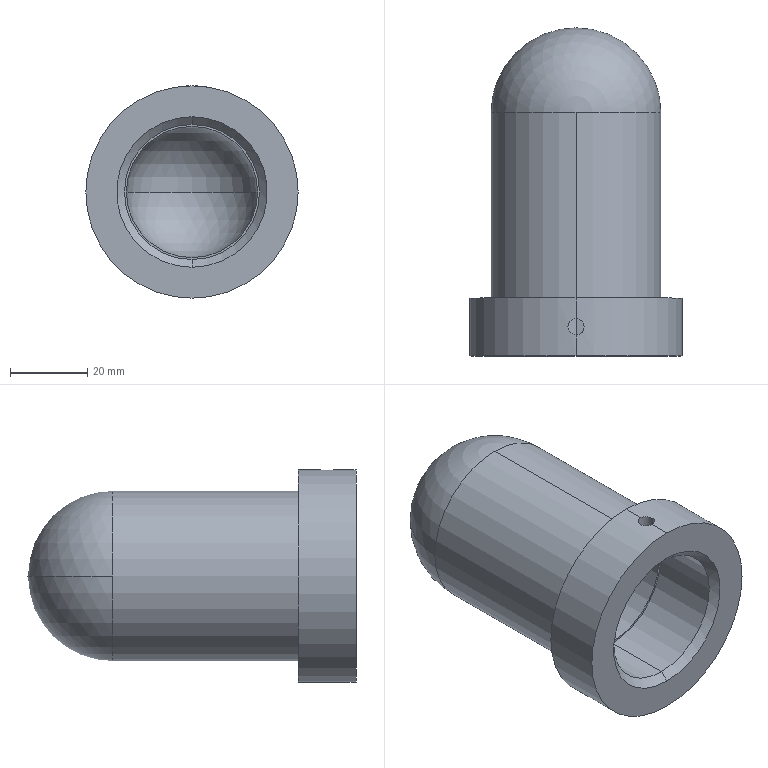Part | SolidWorks | features 3DProfileFeature 1, Chamfer 1, HoleWzd 1, Revolution 1 | 1 solid | 19 faces | box 55 x 85 x 55 mm | volume 61984 mm3 | cylinder 10 | sphere 4 | plane 3 | cone 2 | commonest cylinder face diameters 4.2 x2 34 x2 35 x2 44 x2 55 x2
STEP:
#1=CARTESIAN_POINT('',(0.,2.,17.5));
#2=VERTEX_POINT('',#1);
#3=CARTESIAN_POINT('',(0.,2.,-17.5));
#4=VERTEX_POINT('',#3);
#5=CARTESIAN_POINT('',(0.,2.,0.));
#6=DIRECTION('',(0.,-1.,0.));
#7=DIRECTION('',(0.,0.,1.));
#8=AXIS2_PLACEMENT_3D('',#5,#6,#7);
#9=CIRCLE('',#8,17.5);
#10=EDGE_CURVE('',#2,#4,#9,.T.);
#11=ORIENTED_EDGE('',*,*,#10,.F.);
#12=CARTESIAN_POINT('',(0.,0.,19.5));
#13=VERTEX_POINT('',#12);
#14=CARTESIAN_POINT('',(0.,2.,17.5));
#15=DIRECTION('',(0.,-0.7071,0.7071));
#16=VECTOR('',#15,1000.);
#17=LINE('',#14,#16);
#18=EDGE_CURVE('',#2,#13,#17,.T.);
#19=ORIENTED_EDGE('',*,*,#18,.T.);
#20=CARTESIAN_POINT('',(0.,0.,-19.5));
#21=VERTEX_POINT('',#20);
#22=CARTESIAN_POINT('',(0.,0.,0.));
#23=DIRECTION('',(0.,1.,0.));
#24=DIRECTION('',(0.,0.,1.));
#25=AXIS2_PLACEMENT_3D('',#22,#23,#24);
#26=CIRCLE('',#25,19.5);
#27=EDGE_CURVE('',#21,#13,#26,.T.);
#28=ORIENTED_EDGE('',*,*,#27,.F.);
#29=CARTESIAN_POINT('',(0.,2.,-17.5));
#30=DIRECTION('',(0.,-0.7071,-0.7071));
#31=VECTOR('',#30,1000.);
#32=LINE('',#29,#31);
#33=EDGE_CURVE('',#4,#21,#32,.T.);
#34=ORIENTED_EDGE('',*,*,#33,.F.);
#35=EDGE_LOOP('',(#11,#19,#28,#34));
#36=FACE_OUTER_BOUND('',#35,.T.);
#37=CARTESIAN_POINT('',(0.,2.,0.));
#38=DIRECTION('',(0.,-1.,0.));
#39=DIRECTION('',(0.,0.,-1.));
#40=AXIS2_PLACEMENT_3D('',#37,#38,#39);
#41=CONICAL_SURFACE('',#40,17.5,0.7854);
#42=ADVANCED_FACE('',(#36),#41,.F.);
#43=CARTESIAN_POINT('',(-2.101,7.524,17.373));
#44=VERTEX_POINT('',#43);
#45=CARTESIAN_POINT('',(0.,5.424,17.5));
#46=VERTEX_POINT('',#45);
#47=CARTESIAN_POINT('',(-2.101,7.524,17.373));
#48=CARTESIAN_POINT('',(-2.101,7.25,17.373));
#49=CARTESIAN_POINT('',(-2.046,6.973,17.38));
#50=CARTESIAN_POINT('',(-1.837,6.467,17.404));
#51=CARTESIAN_POINT('',(-1.68,6.233,17.42));
#52=CARTESIAN_POINT('',(-1.389,5.942,17.445));
#53=CARTESIAN_POINT('',(-1.281,5.854,17.453));
#54=CARTESIAN_POINT('',(-1.053,5.701,17.469));
#55=CARTESIAN_POINT('',(-0.9324,5.637,17.476));
#56=CARTESIAN_POINT('',(-0.6779,5.531,17.487));
#57=CARTESIAN_POINT('',(-0.5444,5.491,17.492));
#58=CARTESIAN_POINT('',(-0.2756,5.438,17.498));
#59=CARTESIAN_POINT('',(-0.1389,5.424,17.5));
#60=CARTESIAN_POINT('',(0.,5.424,17.5));
#61=B_SPLINE_CURVE_WITH_KNOTS('',3,(#47,#48,#49,#50,#51,#52,#53,#54,#55,#56,#57,#58,#59,#60),.UNSPECIFIED.,.F.,.F.,(4,2,2,2,2,2,4),(0.006571,0.007393,0.008215,0.008626,0.009037,0.009448,0.009859),.UNSPECIFIED.);
#62=EDGE_CURVE('',#44,#46,#61,.T.);
#63=ORIENTED_EDGE('',*,*,#62,.F.);
#64=CARTESIAN_POINT('',(-2.102,7.524,27.42));
#65=VERTEX_POINT('',#64);
#66=CARTESIAN_POINT('',(-2.102,7.524,27.5));
#67=DIRECTION('',(-0.00007928,0.,1.));
#68=VECTOR('',#67,1000.);
#69=LINE('',#66,#68);
#70=EDGE_CURVE('',#44,#65,#69,.T.);
#71=ORIENTED_EDGE('',*,*,#70,.T.);
#72=CARTESIAN_POINT('',(0.,5.424,27.5));
#73=VERTEX_POINT('',#72);
#74=CARTESIAN_POINT('',(0.,5.424,27.5));
#75=CARTESIAN_POINT('',(-0.1371,5.424,27.5));
#76=CARTESIAN_POINT('',(-0.2763,5.438,27.499));
#77=CARTESIAN_POINT('',(-0.5459,5.491,27.495));
#78=CARTESIAN_POINT('',(-0.6769,5.531,27.492));
#79=CARTESIAN_POINT('',(-0.9314,5.636,27.485));
#80=CARTESIAN_POINT('',(-1.054,5.702,27.48));
#81=CARTESIAN_POINT('',(-1.282,5.854,27.47));
#82=CARTESIAN_POINT('',(-1.388,5.94,27.465));
#83=CARTESIAN_POINT('',(-1.584,6.136,27.454));
#84=CARTESIAN_POINT('',(-1.671,6.243,27.449));
#85=CARTESIAN_POINT('',(-1.824,6.47,27.44));
#86=CARTESIAN_POINT('',(-1.889,6.593,27.435));
#87=CARTESIAN_POINT('',(-1.995,6.847,27.428));
#88=CARTESIAN_POINT('',(-2.035,6.978,27.425));
#89=CARTESIAN_POINT('',(-2.088,7.248,27.421));
#90=CARTESIAN_POINT('',(-2.102,7.387,27.42));
#91=CARTESIAN_POINT('',(-2.102,7.524,27.42));
#92=B_SPLINE_CURVE_WITH_KNOTS('',3,(#74,#75,#76,#77,#78,#79,#80,#81,#82,#83,#84,#85,#86,#87,#88,#89,#90,#91),.UNSPECIFIED.,.F.,.F.,(4,2,2,2,2,2,2,2,4),(0.003283,0.003693,0.004104,0.004515,0.004925,0.005336,0.005747,0.006157,0.006568),.UNSPECIFIED.);
#93=EDGE_CURVE('',#73,#65,#92,.T.);
#94=ORIENTED_EDGE('',*,*,#93,.F.);
#95=CARTESIAN_POINT('',(2.098,7.524,27.42));
#96=VERTEX_POINT('',#95);
#97=CARTESIAN_POINT('',(2.098,7.524,27.42));
#98=CARTESIAN_POINT('',(2.098,7.385,27.42));
#99=CARTESIAN_POINT('',(2.084,7.249,27.421));
#100=CARTESIAN_POINT('',(2.031,6.981,27.425));
#101=CARTESIAN_POINT('',(1.991,6.847,27.428));
#102=CARTESIAN_POINT('',(1.885,6.593,27.435));
#103=CARTESIAN_POINT('',(1.821,6.472,27.44));
#104=CARTESIAN_POINT('',(1.668,6.244,27.449));
#105=CARTESIAN_POINT('',(1.58,6.136,27.455));
#106=CARTESIAN_POINT('',(1.289,5.846,27.47));
#107=CARTESIAN_POINT('',(1.055,5.689,27.481));
#108=CARTESIAN_POINT('',(0.5502,5.48,27.496));
#109=CARTESIAN_POINT('',(0.2739,5.424,27.5));
#110=CARTESIAN_POINT('',(0.,5.424,27.5));
#111=B_SPLINE_CURVE_WITH_KNOTS('',3,(#97,#98,#99,#100,#101,#102,#103,#104,#105,#106,#107,#108,#109,#110),.UNSPECIFIED.,.F.,.F.,(4,2,2,2,2,2,4),(0.,0.0004103,0.0008206,0.001231,0.001641,0.002462,0.003283),.UNSPECIFIED.);
#112=EDGE_CURVE('',#96,#73,#111,.T.);
#113=ORIENTED_EDGE('',*,*,#112,.F.);
#114=CARTESIAN_POINT('',(2.099,7.524,17.374));
#115=VERTEX_POINT('',#114);
#116=CARTESIAN_POINT('',(2.098,7.524,27.5));
#117=DIRECTION('',(-0.00007928,0.,1.));
#118=VECTOR('',#117,1000.);
#119=LINE('',#116,#118);
#120=EDGE_CURVE('',#115,#96,#119,.T.);
#121=ORIENTED_EDGE('',*,*,#120,.F.);
#122=CARTESIAN_POINT('',(0.,5.424,17.5));
#123=CARTESIAN_POINT('',(0.1387,5.424,17.5));
#124=CARTESIAN_POINT('',(0.2751,5.438,17.498));
#125=CARTESIAN_POINT('',(0.5434,5.491,17.492));
#126=CARTESIAN_POINT('',(0.6767,5.532,17.487));
#127=CARTESIAN_POINT('',(0.9306,5.637,17.476));
#128=CARTESIAN_POINT('',(1.051,5.702,17.469));
#129=CARTESIAN_POINT('',(1.279,5.854,17.454));
#130=CARTESIAN_POINT('',(1.387,5.943,17.445));
#131=CARTESIAN_POINT('',(1.677,6.233,17.421));
#132=CARTESIAN_POINT('',(1.833,6.466,17.404));
#133=CARTESIAN_POINT('',(2.043,6.971,17.381));
#134=CARTESIAN_POINT('',(2.099,7.247,17.374));
#135=CARTESIAN_POINT('',(2.099,7.524,17.374));
#136=B_SPLINE_CURVE_WITH_KNOTS('',3,(#122,#123,#124,#125,#126,#127,#128,#129,#130,#131,#132,#133,#134,#135),.UNSPECIFIED.,.F.,.F.,(4,2,2,2,2,2,4),(0.009859,0.01027,0.01068,0.01109,0.0115,0.01232,0.01314),.UNSPECIFIED.);
#137=EDGE_CURVE('',#46,#115,#136,.T.);
#138=ORIENTED_EDGE('',*,*,#137,.F.);
#139=EDGE_LOOP('',(#63,#71,#94,#113,#121,#138));
#140=FACE_OUTER_BOUND('',#139,.T.);
#141=CARTESIAN_POINT('',(-0.00218,7.524,27.5));
#142=DIRECTION('',(-0.00007928,0.,1.));
#143=DIRECTION('',(1.,0.,0.00007928));
#144=AXIS2_PLACEMENT_3D('',#141,#142,#143);
#145=CYLINDRICAL_SURFACE('',#144,2.1);
#146=ADVANCED_FACE('',(#140),#145,.F.);
#147=CARTESIAN_POINT('',(0.,80.,0.));
#148=VERTEX_POINT('',#147);
#149=CARTESIAN_POINT('',(-17.,63.,0.));
#150=VERTEX_POINT('',#149);
#151=CARTESIAN_POINT('',(0.,63.,0.));
#152=DIRECTION('',(0.,0.,1.));
#153=DIRECTION('',(1.,0.,0.));
#154=AXIS2_PLACEMENT_3D('',#151,#152,#153);
#155=CIRCLE('',#154,17.);
#156=EDGE_CURVE('',#148,#150,#155,.T.);
#157=ORIENTED_EDGE('',*,*,#156,.F.);
#158=CARTESIAN_POINT('',(17.,63.,0.));
#159=VERTEX_POINT('',#158);
#160=CARTESIAN_POINT('',(0.,63.,0.));
#161=DIRECTION('',(0.,0.,-1.));
#162=DIRECTION('',(-1.,0.,0.));
#163=AXIS2_PLACEMENT_3D('',#160,#161,#162);
#164=CIRCLE('',#163,17.);
#165=EDGE_CURVE('',#148,#159,#164,.T.);
#166=ORIENTED_EDGE('',*,*,#165,.T.);
#167=CARTESIAN_POINT('',(0.,63.,17.));
#168=VERTEX_POINT('',#167);
#169=CARTESIAN_POINT('',(0.,63.,0.));
#170=DIRECTION('',(0.,-1.,0.));
#171=DIRECTION('',(0.,0.,-1.));
#172=AXIS2_PLACEMENT_3D('',#169,#170,#171);
#173=CIRCLE('',#172,17.);
#174=EDGE_CURVE('',#159,#168,#173,.T.);
#175=ORIENTED_EDGE('',*,*,#174,.T.);
#176=CARTESIAN_POINT('',(0.,63.,0.));
#177=DIRECTION('',(0.,-1.,0.));
#178=DIRECTION('',(0.,0.,-1.));
#179=AXIS2_PLACEMENT_3D('',#176,#177,#178);
#180=CIRCLE('',#179,17.);
#181=EDGE_CURVE('',#168,#150,#180,.T.);
#182=ORIENTED_EDGE('',*,*,#181,.T.);
#183=EDGE_LOOP('',(#157,#166,#175,#182));
#184=FACE_OUTER_BOUND('',#183,.T.);
#185=CARTESIAN_POINT('',(0.,63.,0.));
#186=DIRECTION('',(0.,0.,-1.));
#187=DIRECTION('',(-1.,0.,0.));
#188=AXIS2_PLACEMENT_3D('',#185,#186,#187);
#189=SPHERICAL_SURFACE('',#188,17.);
#190=ADVANCED_FACE('',(#184),#189,.F.);
#191=ORIENTED_EDGE('',*,*,#181,.F.);
#192=CARTESIAN_POINT('',(0.,20.,17.));
#193=VERTEX_POINT('',#192);
#194=CARTESIAN_POINT('',(0.,0.,17.));
#195=DIRECTION('',(0.,-1.,0.));
#196=VECTOR('',#195,1000.);
#197=LINE('',#194,#196);
#198=EDGE_CURVE('',#168,#193,#197,.T.);
#199=ORIENTED_EDGE('',*,*,#198,.T.);
#200=CARTESIAN_POINT('',(0.,20.,-17.));
#201=VERTEX_POINT('',#200);
#202=CARTESIAN_POINT('',(0.,20.,0.));
#203=DIRECTION('',(0.,-1.,0.));
#204=DIRECTION('',(0.,0.,-1.));
#205=AXIS2_PLACEMENT_3D('',#202,#203,#204);
#206=CIRCLE('',#205,17.);
#207=EDGE_CURVE('',#193,#201,#206,.T.);
#208=ORIENTED_EDGE('',*,*,#207,.T.);
#209=CARTESIAN_POINT('',(0.,63.,-17.));
#210=VERTEX_POINT('',#209);
#211=CARTESIAN_POINT('',(0.,0.,-17.));
#212=DIRECTION('',(0.,-1.,0.));
#213=VECTOR('',#212,1000.);
#214=LINE('',#211,#213);
#215=EDGE_CURVE('',#210,#201,#214,.T.);
#216=ORIENTED_EDGE('',*,*,#215,.F.);
#217=CARTESIAN_POINT('',(0.,63.,0.));
#218=DIRECTION('',(0.,-1.,0.));
#219=DIRECTION('',(0.,0.,-1.));
#220=AXIS2_PLACEMENT_3D('',#217,#218,#219);
#221=CIRCLE('',#220,17.);
#222=EDGE_CURVE('',#150,#210,#221,.T.);
#223=ORIENTED_EDGE('',*,*,#222,.F.);
#224=EDGE_LOOP('',(#191,#199,#208,#216,#223));
#225=FACE_OUTER_BOUND('',#224,.T.);
#226=CARTESIAN_POINT('',(0.,0.,0.));
#227=DIRECTION('',(0.,-1.,0.));
#228=DIRECTION('',(0.,0.,-1.));
#229=AXIS2_PLACEMENT_3D('',#226,#227,#228);
#230=CYLINDRICAL_SURFACE('',#229,17.);
#231=ADVANCED_FACE('',(#225),#230,.F.);
#232=CARTESIAN_POINT('',(0.,20.,17.5));
#233=VERTEX_POINT('',#232);
#234=CARTESIAN_POINT('',(0.,20.,-17.5));
#235=VERTEX_POINT('',#234);
#236=CARTESIAN_POINT('',(0.,20.,0.));
#237=DIRECTION('',(0.,-1.,0.));
#238=DIRECTION('',(0.,0.,-1.));
#239=AXIS2_PLACEMENT_3D('',#236,#237,#238);
#240=CIRCLE('',#239,17.5);
#241=EDGE_CURVE('',#233,#235,#240,.T.);
#242=ORIENTED_EDGE('',*,*,#241,.F.);
#243=CARTESIAN_POINT('',(0.,9.624,17.5));
#244=VERTEX_POINT('',#243);
#245=CARTESIAN_POINT('',(0.,0.,17.5));
#246=DIRECTION('',(0.,-1.,0.));
#247=VECTOR('',#246,1000.);
#248=LINE('',#245,#247);
#249=EDGE_CURVE('',#233,#244,#248,.T.);
#250=ORIENTED_EDGE('',*,*,#249,.T.);
#251=CARTESIAN_POINT('',(0.,9.624,17.5));
#252=CARTESIAN_POINT('',(-0.1371,9.624,17.5));
#253=CARTESIAN_POINT('',(-0.2764,9.611,17.498));
#254=CARTESIAN_POINT('',(-0.5459,9.557,17.492));
#255=CARTESIAN_POINT('',(-0.677,9.517,17.487));
#256=CARTESIAN_POINT('',(-0.9314,9.412,17.476));
#257=CARTESIAN_POINT('',(-1.054,9.346,17.469));
#258=CARTESIAN_POINT('',(-1.282,9.194,17.453));
#259=CARTESIAN_POINT('',(-1.388,9.107,17.445));
#260=CARTESIAN_POINT('',(-1.584,8.912,17.428));
#261=CARTESIAN_POINT('',(-1.671,8.806,17.42));
#262=CARTESIAN_POINT('',(-1.823,8.578,17.405));
#263=CARTESIAN_POINT('',(-1.889,8.455,17.398));
#264=CARTESIAN_POINT('',(-1.994,8.201,17.386));
#265=CARTESIAN_POINT('',(-2.034,8.07,17.381));
#266=CARTESIAN_POINT('',(-2.088,7.801,17.375));
#267=CARTESIAN_POINT('',(-2.101,7.661,17.373));
#268=CARTESIAN_POINT('',(-2.101,7.524,17.373));
#269=B_SPLINE_CURVE_WITH_KNOTS('',3,(#251,#252,#253,#254,#255,#256,#257,#258,#259,#260,#261,#262,#263,#264,#265,#266,#267,#268),.UNSPECIFIED.,.F.,.F.,(4,2,2,2,2,2,2,2,4),(0.003285,0.003696,0.004107,0.004518,0.004928,0.005339,0.00575,0.006161,0.006571),.UNSPECIFIED.);
#270=EDGE_CURVE('',#244,#44,#269,.T.);
#271=ORIENTED_EDGE('',*,*,#270,.T.);
#272=ORIENTED_EDGE('',*,*,#62,.T.);
#273=CARTESIAN_POINT('',(0.,0.,17.5));
#274=DIRECTION('',(0.,-1.,0.));
#275=VECTOR('',#274,1000.);
#276=LINE('',#273,#275);
#277=EDGE_CURVE('',#46,#2,#276,.T.);
#278=ORIENTED_EDGE('',*,*,#277,.T.);
#279=ORIENTED_EDGE('',*,*,#10,.T.);
#280=CARTESIAN_POINT('',(0.,0.,-17.5));
#281=DIRECTION('',(0.,-1.,0.));
#282=VECTOR('',#281,1000.);
#283=LINE('',#280,#282);
#284=EDGE_CURVE('',#235,#4,#283,.T.);
#285=ORIENTED_EDGE('',*,*,#284,.F.);
#286=EDGE_LOOP('',(#242,#250,#271,#272,#278,#279,#285));
#287=FACE_OUTER_BOUND('',#286,.T.);
#288=CARTESIAN_POINT('',(0.,0.,0.));
#289=DIRECTION('',(0.,-1.,0.));
#290=DIRECTION('',(0.,0.,-1.));
#291=AXIS2_PLACEMENT_3D('',#288,#289,#290);
#292=CYLINDRICAL_SURFACE('',#291,17.5);
#293=ADVANCED_FACE('',(#287),#292,.F.);
#294=CARTESIAN_POINT('',(0.,15.,-27.5));
#295=VERTEX_POINT('',#294);
#296=CARTESIAN_POINT('',(0.,15.,27.5));
#297=VERTEX_POINT('',#296);
#298=CARTESIAN_POINT('',(0.,15.,0.));
#299=DIRECTION('',(0.,-1.,0.));
#300=DIRECTION('',(0.,0.,-1.));
#301=AXIS2_PLACEMENT_3D('',#298,#299,#300);
#302=CIRCLE('',#301,27.5);
#303=EDGE_CURVE('',#295,#297,#302,.T.);
#304=ORIENTED_EDGE('',*,*,#303,.T.);
#305=CARTESIAN_POINT('',(0.,9.624,27.5));
#306=VERTEX_POINT('',#305);
#307=CARTESIAN_POINT('',(0.,0.,27.5));
#308=DIRECTION('',(0.,-1.,0.));
#309=VECTOR('',#308,1000.);
#310=LINE('',#307,#309);
#311=EDGE_CURVE('',#297,#306,#310,.T.);
#312=ORIENTED_EDGE('',*,*,#311,.T.);
#313=CARTESIAN_POINT('',(0.,9.624,27.5));
#314=CARTESIAN_POINT('',(0.1385,9.624,27.5));
#315=CARTESIAN_POINT('',(0.2751,9.61,27.499));
#316=CARTESIAN_POINT('',(0.5431,9.557,27.495));
#317=CARTESIAN_POINT('',(0.6762,9.516,27.492));
#318=CARTESIAN_POINT('',(0.9302,9.411,27.485));
#319=CARTESIAN_POINT('',(1.051,9.346,27.48));
#320=CARTESIAN_POINT('',(1.278,9.194,27.471));
#321=CARTESIAN_POINT('',(1.386,9.106,27.465));
#322=CARTESIAN_POINT('',(1.58,8.912,27.455));
#323=CARTESIAN_POINT('',(1.667,8.807,27.45));
#324=CARTESIAN_POINT('',(1.82,8.577,27.44));
#325=CARTESIAN_POINT('',(1.885,8.455,27.435));
#326=CARTESIAN_POINT('',(2.042,8.077,27.424));
#327=CARTESIAN_POINT('',(2.098,7.801,27.42));
#328=CARTESIAN_POINT('',(2.098,7.524,27.42));
#329=B_SPLINE_CURVE_WITH_KNOTS('',3,(#313,#314,#315,#316,#317,#318,#319,#320,#321,#322,#323,#324,#325,#326,#327,#328),.UNSPECIFIED.,.F.,.F.,(4,2,2,2,2,2,2,4),(0.009855,0.01026,0.01067,0.01108,0.01149,0.0119,0.01231,0.01313),.UNSPECIFIED.);
#330=EDGE_CURVE('',#306,#96,#329,.T.);
#331=ORIENTED_EDGE('',*,*,#330,.T.);
#332=ORIENTED_EDGE('',*,*,#112,.T.);
#333=CARTESIAN_POINT('',(0.,0.,27.5));
#334=VERTEX_POINT('',#333);
#335=CARTESIAN_POINT('',(0.,0.,27.5));
#336=DIRECTION('',(0.,-1.,0.));
#337=VECTOR('',#336,1000.);
#338=LINE('',#335,#337);
#339=EDGE_CURVE('',#73,#334,#338,.T.);
#340=ORIENTED_EDGE('',*,*,#339,.T.);
#341=CARTESIAN_POINT('',(0.,0.,-27.5));
#342=VERTEX_POINT('',#341);
#343=CARTESIAN_POINT('',(0.,0.,0.));
#344=DIRECTION('',(0.,-1.,0.));
#345=DIRECTION('',(0.,0.,-1.));
#346=AXIS2_PLACEMENT_3D('',#343,#344,#345);
#347=CIRCLE('',#346,27.5);
#348=EDGE_CURVE('',#342,#334,#347,.T.);
#349=ORIENTED_EDGE('',*,*,#348,.F.);
#350=CARTESIAN_POINT('',(0.,0.,-27.5));
#351=DIRECTION('',(0.,-1.,0.));
#352=VECTOR('',#351,1000.);
#353=LINE('',#350,#352);
#354=EDGE_CURVE('',#295,#342,#353,.T.);
#355=ORIENTED_EDGE('',*,*,#354,.F.);
#356=EDGE_LOOP('',(#304,#312,#331,#332,#340,#349,#355));
#357=FACE_OUTER_BOUND('',#356,.T.);
#358=CARTESIAN_POINT('',(0.,0.,0.));
#359=DIRECTION('',(0.,-1.,0.));
#360=DIRECTION('',(0.,0.,-1.));
#361=AXIS2_PLACEMENT_3D('',#358,#359,#360);
#362=CYLINDRICAL_SURFACE('',#361,27.5);
#363=ADVANCED_FACE('',(#357),#362,.T.);
#364=CARTESIAN_POINT('',(22.,63.,0.));
#365=VERTEX_POINT('',#364);
#366=CARTESIAN_POINT('',(0.,63.,22.));
#367=VERTEX_POINT('',#366);
#368=CARTESIAN_POINT('',(0.,63.,0.));
#369=DIRECTION('',(0.,-1.,0.));
#370=DIRECTION('',(0.,0.,-1.));
#371=AXIS2_PLACEMENT_3D('',#368,#369,#370);
#372=CIRCLE('',#371,22.);
#373=EDGE_CURVE('',#365,#367,#372,.T.);
#374=ORIENTED_EDGE('',*,*,#373,.T.);
#375=CARTESIAN_POINT('',(0.,15.,22.));
#376=VERTEX_POINT('',#375);
#377=CARTESIAN_POINT('',(0.,0.,22.));
#378=DIRECTION('',(0.,-1.,0.));
#379=VECTOR('',#378,1000.);
#380=LINE('',#377,#379);
#381=EDGE_CURVE('',#367,#376,#380,.T.);
#382=ORIENTED_EDGE('',*,*,#381,.T.);
#383=CARTESIAN_POINT('',(0.,15.,-22.));
#384=VERTEX_POINT('',#383);
#385=CARTESIAN_POINT('',(0.,15.,0.));
#386=DIRECTION('',(0.,-1.,0.));
#387=DIRECTION('',(0.,0.,-1.));
#388=AXIS2_PLACEMENT_3D('',#385,#386,#387);
#389=CIRCLE('',#388,22.);
#390=EDGE_CURVE('',#384,#376,#389,.T.);
#391=ORIENTED_EDGE('',*,*,#390,.F.);
#392=CARTESIAN_POINT('',(0.,63.,-22.));
#393=VERTEX_POINT('',#392);
#394=CARTESIAN_POINT('',(0.,0.,-22.));
#395=DIRECTION('',(0.,-1.,0.));
#396=VECTOR('',#395,1000.);
#397=LINE('',#394,#396);
#398=EDGE_CURVE('',#393,#384,#397,.T.);
#399=ORIENTED_EDGE('',*,*,#398,.F.);
#400=CARTESIAN_POINT('',(0.,63.,0.));
#401=DIRECTION('',(0.,-1.,0.));
#402=DIRECTION('',(0.,0.,-1.));
#403=AXIS2_PLACEMENT_3D('',#400,#401,#402);
#404=CIRCLE('',#403,22.);
#405=EDGE_CURVE('',#393,#365,#404,.T.);
#406=ORIENTED_EDGE('',*,*,#405,.T.);
#407=EDGE_LOOP('',(#374,#382,#391,#399,#406));
#408=FACE_OUTER_BOUND('',#407,.T.);
#409=CARTESIAN_POINT('',(0.,0.,0.));
#410=DIRECTION('',(0.,-1.,0.));
#411=DIRECTION('',(0.,0.,-1.));
#412=AXIS2_PLACEMENT_3D('',#409,#410,#411);
#413=CYLINDRICAL_SURFACE('',#412,22.);
#414=ADVANCED_FACE('',(#408),#413,.T.);
#415=CARTESIAN_POINT('',(0.,85.,0.));
#416=VERTEX_POINT('',#415);
#417=CARTESIAN_POINT('',(-22.,63.,0.));
#418=VERTEX_POINT('',#417);
#419=CARTESIAN_POINT('',(0.,63.,0.));
#420=DIRECTION('',(0.,0.,1.));
#421=DIRECTION('',(1.,0.,0.));
#422=AXIS2_PLACEMENT_3D('',#419,#420,#421);
#423=CIRCLE('',#422,22.);
#424=EDGE_CURVE('',#416,#418,#423,.T.);
#425=ORIENTED_EDGE('',*,*,#424,.F.);
#426=CARTESIAN_POINT('',(0.,63.,0.));
#427=DIRECTION('',(0.,0.,-1.));
#428=DIRECTION('',(-1.,0.,0.));
#429=AXIS2_PLACEMENT_3D('',#426,#427,#428);
#430=CIRCLE('',#429,22.);
#431=EDGE_CURVE('',#416,#365,#430,.T.);
#432=ORIENTED_EDGE('',*,*,#431,.T.);
#433=ORIENTED_EDGE('',*,*,#405,.F.);
#434=CARTESIAN_POINT('',(0.,63.,0.));
#435=DIRECTION('',(0.,-1.,0.));
#436=DIRECTION('',(0.,0.,-1.));
#437=AXIS2_PLACEMENT_3D('',#434,#435,#436);
#438=CIRCLE('',#437,22.);
#439=EDGE_CURVE('',#418,#393,#438,.T.);
#440=ORIENTED_EDGE('',*,*,#439,.F.);
#441=EDGE_LOOP('',(#425,#432,#433,#440));
#442=FACE_OUTER_BOUND('',#441,.T.);
#443=CARTESIAN_POINT('',(0.,63.,0.));
#444=DIRECTION('',(0.,0.,-1.));
#445=DIRECTION('',(-1.,0.,0.));
#446=AXIS2_PLACEMENT_3D('',#443,#444,#445);
#447=SPHERICAL_SURFACE('',#446,22.);
#448=ADVANCED_FACE('',(#442),#447,.T.);
#449=ORIENTED_EDGE('',*,*,#431,.F.);
#450=ORIENTED_EDGE('',*,*,#424,.T.);
#451=CARTESIAN_POINT('',(0.,63.,0.));
#452=DIRECTION('',(0.,-1.,0.));
#453=DIRECTION('',(0.,0.,-1.));
#454=AXIS2_PLACEMENT_3D('',#451,#452,#453);
#455=CIRCLE('',#454,22.);
#456=EDGE_CURVE('',#367,#418,#455,.T.);
#457=ORIENTED_EDGE('',*,*,#456,.F.);
#458=ORIENTED_EDGE('',*,*,#373,.F.);
#459=EDGE_LOOP('',(#449,#450,#457,#458));
#460=FACE_OUTER_BOUND('',#459,.T.);
#461=CARTESIAN_POINT('',(0.,63.,0.));
#462=DIRECTION('',(0.,0.,-1.));
#463=DIRECTION('',(-1.,0.,0.));
#464=AXIS2_PLACEMENT_3D('',#461,#462,#463);
#465=SPHERICAL_SURFACE('',#464,22.);
#466=ADVANCED_FACE('',(#460),#465,.T.);
#467=ORIENTED_EDGE('',*,*,#381,.F.);
#468=ORIENTED_EDGE('',*,*,#456,.T.);
#469=ORIENTED_EDGE('',*,*,#439,.T.);
#470=ORIENTED_EDGE('',*,*,#398,.T.);
#471=CARTESIAN_POINT('',(0.,15.,0.));
#472=DIRECTION('',(0.,-1.,0.));
#473=DIRECTION('',(0.,0.,-1.));
#474=AXIS2_PLACEMENT_3D('',#471,#472,#473);
#475=CIRCLE('',#474,22.);
#476=EDGE_CURVE('',#376,#384,#475,.T.);
#477=ORIENTED_EDGE('',*,*,#476,.F.);
#478=EDGE_LOOP('',(#467,#468,#469,#470,#477));
#479=FACE_OUTER_BOUND('',#478,.T.);
#480=CARTESIAN_POINT('',(0.,0.,0.));
#481=DIRECTION('',(0.,-1.,0.));
#482=DIRECTION('',(0.,0.,-1.));
#483=AXIS2_PLACEMENT_3D('',#480,#481,#482);
#484=CYLINDRICAL_SURFACE('',#483,22.);
#485=ADVANCED_FACE('',(#479),#484,.T.);
#486=ORIENTED_EDGE('',*,*,#303,.F.);
#487=CARTESIAN_POINT('',(0.,15.,0.));
#488=DIRECTION('',(0.,-1.,0.));
#489=DIRECTION('',(0.,0.,-1.));
#490=AXIS2_PLACEMENT_3D('',#487,#488,#489);
#491=CIRCLE('',#490,27.5);
#492=EDGE_CURVE('',#297,#295,#491,.T.);
#493=ORIENTED_EDGE('',*,*,#492,.F.);
#494=EDGE_LOOP('',(#486,#493));
#495=FACE_OUTER_BOUND('',#494,.T.);
#496=ORIENTED_EDGE('',*,*,#390,.T.);
#497=ORIENTED_EDGE('',*,*,#476,.T.);
#498=EDGE_LOOP('',(#496,#497));
#499=FACE_BOUND('',#498,.T.);
#500=CARTESIAN_POINT('',(-22.,15.,0.));
#501=DIRECTION('',(0.,-1.,0.));
#502=DIRECTION('',(0.,0.,-1.));
#503=AXIS2_PLACEMENT_3D('',#500,#501,#502);
#504=PLANE('',#503);
#505=ADVANCED_FACE('',(#495,#499),#504,.F.);
#506=ORIENTED_EDGE('',*,*,#311,.F.);
#507=ORIENTED_EDGE('',*,*,#492,.T.);
#508=ORIENTED_EDGE('',*,*,#354,.T.);
#509=CARTESIAN_POINT('',(0.,0.,0.));
#510=DIRECTION('',(0.,-1.,0.));
#511=DIRECTION('',(0.,0.,-1.));
#512=AXIS2_PLACEMENT_3D('',#509,#510,#511);
#513=CIRCLE('',#512,27.5);
#514=EDGE_CURVE('',#334,#342,#513,.T.);
#515=ORIENTED_EDGE('',*,*,#514,.F.);
#516=ORIENTED_EDGE('',*,*,#339,.F.);
#517=ORIENTED_EDGE('',*,*,#93,.T.);
#518=CARTESIAN_POINT('',(-2.102,7.524,27.42));
#519=CARTESIAN_POINT('',(-2.102,7.799,27.42));
#520=CARTESIAN_POINT('',(-2.047,8.075,27.424));
#521=CARTESIAN_POINT('',(-1.837,8.581,27.439));
#522=CARTESIAN_POINT('',(-1.681,8.816,27.449));
#523=CARTESIAN_POINT('',(-1.39,9.106,27.465));
#524=CARTESIAN_POINT('',(-1.282,9.195,27.47));
#525=CARTESIAN_POINT('',(-1.053,9.347,27.48));
#526=CARTESIAN_POINT('',(-0.9323,9.412,27.484));
#527=CARTESIAN_POINT('',(-0.6779,9.517,27.492));
#528=CARTESIAN_POINT('',(-0.5442,9.558,27.495));
#529=CARTESIAN_POINT('',(-0.2754,9.611,27.499));
#530=CARTESIAN_POINT('',(-0.1388,9.624,27.5));
#531=CARTESIAN_POINT('',(0.,9.624,27.5));
#532=B_SPLINE_CURVE_WITH_KNOTS('',3,(#518,#519,#520,#521,#522,#523,#524,#525,#526,#527,#528,#529,#530,#531),.UNSPECIFIED.,.F.,.F.,(4,2,2,2,2,2,4),(0.006568,0.00739,0.008211,0.008622,0.009033,0.009444,0.009855),.UNSPECIFIED.);
#533=EDGE_CURVE('',#65,#306,#532,.T.);
#534=ORIENTED_EDGE('',*,*,#533,.T.);
#535=EDGE_LOOP('',(#506,#507,#508,#515,#516,#517,#534));
#536=FACE_OUTER_BOUND('',#535,.T.);
#537=CARTESIAN_POINT('',(0.,0.,0.));
#538=DIRECTION('',(0.,-1.,0.));
#539=DIRECTION('',(0.,0.,-1.));
#540=AXIS2_PLACEMENT_3D('',#537,#538,#539);
#541=CYLINDRICAL_SURFACE('',#540,27.5);
#542=ADVANCED_FACE('',(#536),#541,.T.);
#543=ORIENTED_EDGE('',*,*,#27,.T.);
#544=CARTESIAN_POINT('',(0.,0.,0.));
#545=DIRECTION('',(0.,1.,0.));
#546=DIRECTION('',(0.,0.,1.));
#547=AXIS2_PLACEMENT_3D('',#544,#545,#546);
#548=CIRCLE('',#547,19.5);
#549=EDGE_CURVE('',#13,#21,#548,.T.);
#550=ORIENTED_EDGE('',*,*,#549,.T.);
#551=EDGE_LOOP('',(#543,#550));
#552=FACE_BOUND('',#551,.T.);
#553=ORIENTED_EDGE('',*,*,#348,.T.);
#554=ORIENTED_EDGE('',*,*,#514,.T.);
#555=EDGE_LOOP('',(#553,#554));
#556=FACE_OUTER_BOUND('',#555,.T.);
#557=CARTESIAN_POINT('',(-27.5,0.,0.));
#558=DIRECTION('',(0.,1.,0.));
#559=DIRECTION('',(0.,0.,1.));
#560=AXIS2_PLACEMENT_3D('',#557,#558,#559);
#561=PLANE('',#560);
#562=ADVANCED_FACE('',(#552,#556),#561,.F.);
#563=ORIENTED_EDGE('',*,*,#249,.F.);
#564=CARTESIAN_POINT('',(0.,20.,0.));
#565=DIRECTION('',(0.,-1.,0.));
#566=DIRECTION('',(0.,0.,-1.));
#567=AXIS2_PLACEMENT_3D('',#564,#565,#566);
#568=CIRCLE('',#567,17.5);
#569=EDGE_CURVE('',#235,#233,#568,.T.);
#570=ORIENTED_EDGE('',*,*,#569,.F.);
#571=ORIENTED_EDGE('',*,*,#284,.T.);
#572=CARTESIAN_POINT('',(0.,2.,0.));
#573=DIRECTION('',(0.,-1.,0.));
#574=DIRECTION('',(0.,0.,1.));
#575=AXIS2_PLACEMENT_3D('',#572,#573,#574);
#576=CIRCLE('',#575,17.5);
#577=EDGE_CURVE('',#4,#2,#576,.T.);
#578=ORIENTED_EDGE('',*,*,#577,.T.);
#579=ORIENTED_EDGE('',*,*,#277,.F.);
#580=ORIENTED_EDGE('',*,*,#137,.T.);
#581=CARTESIAN_POINT('',(2.099,7.524,17.374));
#582=CARTESIAN_POINT('',(2.099,7.663,17.374));
#583=CARTESIAN_POINT('',(2.085,7.8,17.375));
#584=CARTESIAN_POINT('',(2.032,8.068,17.382));
#585=CARTESIAN_POINT('',(1.991,8.202,17.386));
#586=CARTESIAN_POINT('',(1.886,8.456,17.398));
#587=CARTESIAN_POINT('',(1.821,8.576,17.405));
#588=CARTESIAN_POINT('',(1.669,8.804,17.42));
#589=CARTESIAN_POINT('',(1.58,8.912,17.429));
#590=CARTESIAN_POINT('',(1.29,9.203,17.453));
#591=CARTESIAN_POINT('',(1.056,9.359,17.47));
#592=CARTESIAN_POINT('',(0.5507,9.569,17.493));
#593=CARTESIAN_POINT('',(0.2742,9.624,17.5));
#594=CARTESIAN_POINT('',(0.,9.624,17.5));
#595=B_SPLINE_CURVE_WITH_KNOTS('',3,(#581,#582,#583,#584,#585,#586,#587,#588,#589,#590,#591,#592,#593,#594),.UNSPECIFIED.,.F.,.F.,(4,2,2,2,2,2,4),(0.,0.0004106,0.0008213,0.001232,0.001643,0.002464,0.003285),.UNSPECIFIED.);
#596=EDGE_CURVE('',#115,#244,#595,.T.);
#597=ORIENTED_EDGE('',*,*,#596,.T.);
#598=EDGE_LOOP('',(#563,#570,#571,#578,#579,#580,#597));
#599=FACE_OUTER_BOUND('',#598,.T.);
#600=CARTESIAN_POINT('',(0.,0.,0.));
#601=DIRECTION('',(0.,-1.,0.));
#602=DIRECTION('',(0.,0.,-1.));
#603=AXIS2_PLACEMENT_3D('',#600,#601,#602);
#604=CYLINDRICAL_SURFACE('',#603,17.5);
#605=ADVANCED_FACE('',(#599),#604,.F.);
#606=CARTESIAN_POINT('',(0.,20.,0.));
#607=DIRECTION('',(0.,-1.,0.));
#608=DIRECTION('',(0.,0.,-1.));
#609=AXIS2_PLACEMENT_3D('',#606,#607,#608);
#610=CIRCLE('',#609,17.);
#611=EDGE_CURVE('',#201,#193,#610,.T.);
#612=ORIENTED_EDGE('',*,*,#611,.F.);
#613=ORIENTED_EDGE('',*,*,#207,.F.);
#614=EDGE_LOOP('',(#612,#613));
#615=FACE_BOUND('',#614,.T.);
#616=ORIENTED_EDGE('',*,*,#569,.T.);
#617=ORIENTED_EDGE('',*,*,#241,.T.);
#618=EDGE_LOOP('',(#616,#617));
#619=FACE_OUTER_BOUND('',#618,.T.);
#620=CARTESIAN_POINT('',(-17.,20.,0.));
#621=DIRECTION('',(0.,1.,0.));
#622=DIRECTION('',(0.,0.,1.));
#623=AXIS2_PLACEMENT_3D('',#620,#621,#622);
#624=PLANE('',#623);
#625=ADVANCED_FACE('',(#615,#619),#624,.F.);
#626=ORIENTED_EDGE('',*,*,#198,.F.);
#627=ORIENTED_EDGE('',*,*,#174,.F.);
#628=CARTESIAN_POINT('',(0.,63.,0.));
#629=DIRECTION('',(0.,-1.,0.));
#630=DIRECTION('',(0.,0.,-1.));
#631=AXIS2_PLACEMENT_3D('',#628,#629,#630);
#632=CIRCLE('',#631,17.);
#633=EDGE_CURVE('',#210,#159,#632,.T.);
#634=ORIENTED_EDGE('',*,*,#633,.F.);
#635=ORIENTED_EDGE('',*,*,#215,.T.);
#636=ORIENTED_EDGE('',*,*,#611,.T.);
#637=EDGE_LOOP('',(#626,#627,#634,#635,#636));
#638=FACE_OUTER_BOUND('',#637,.T.);
#639=CARTESIAN_POINT('',(0.,0.,0.));
#640=DIRECTION('',(0.,-1.,0.));
#641=DIRECTION('',(0.,0.,-1.));
#642=AXIS2_PLACEMENT_3D('',#639,#640,#641);
#643=CYLINDRICAL_SURFACE('',#642,17.);
#644=ADVANCED_FACE('',(#638),#643,.F.);
#645=ORIENTED_EDGE('',*,*,#165,.F.);
#646=ORIENTED_EDGE('',*,*,#156,.T.);
#647=ORIENTED_EDGE('',*,*,#222,.T.);
#648=ORIENTED_EDGE('',*,*,#633,.T.);
#649=EDGE_LOOP('',(#645,#646,#647,#648));
#650=FACE_OUTER_BOUND('',#649,.T.);
#651=CARTESIAN_POINT('',(0.,63.,0.));
#652=DIRECTION('',(0.,0.,-1.));
#653=DIRECTION('',(-1.,0.,0.));
#654=AXIS2_PLACEMENT_3D('',#651,#652,#653);
#655=SPHERICAL_SURFACE('',#654,17.);
#656=ADVANCED_FACE('',(#650),#655,.F.);
#657=ORIENTED_EDGE('',*,*,#70,.F.);
#658=ORIENTED_EDGE('',*,*,#270,.F.);
#659=ORIENTED_EDGE('',*,*,#596,.F.);
#660=ORIENTED_EDGE('',*,*,#120,.T.);
#661=ORIENTED_EDGE('',*,*,#330,.F.);
#662=ORIENTED_EDGE('',*,*,#533,.F.);
#663=EDGE_LOOP('',(#657,#658,#659,#660,#661,#662));
#664=FACE_OUTER_BOUND('',#663,.T.);
#665=CARTESIAN_POINT('',(-0.00218,7.524,27.5));
#666=DIRECTION('',(-0.00007928,0.,1.));
#667=DIRECTION('',(1.,0.,0.00007928));
#668=AXIS2_PLACEMENT_3D('',#665,#666,#667);
#669=CYLINDRICAL_SURFACE('',#668,2.1);
#670=ADVANCED_FACE('',(#664),#669,.F.);
#671=ORIENTED_EDGE('',*,*,#18,.F.);
#672=ORIENTED_EDGE('',*,*,#577,.F.);
#673=ORIENTED_EDGE('',*,*,#33,.T.);
#674=ORIENTED_EDGE('',*,*,#549,.F.);
#675=EDGE_LOOP('',(#671,#672,#673,#674));
#676=FACE_OUTER_BOUND('',#675,.T.);
#677=CARTESIAN_POINT('',(0.,2.,0.));
#678=DIRECTION('',(0.,-1.,0.));
#679=DIRECTION('',(0.,0.,-1.));
#680=AXIS2_PLACEMENT_3D('',#677,#678,#679);
#681=CONICAL_SURFACE('',#680,17.5,0.7854);
#682=ADVANCED_FACE('',(#676),#681,.F.);
#683=CLOSED_SHELL('',(#42,#146,#190,#231,#293,#363,#414,#448,#466,#485,#505,#542,#562,#605,#625,#644,#656,#670,#682));
#684=MANIFOLD_SOLID_BREP('',#683);
#685=CARTESIAN_POINT('',(0.,0.,0.));
#686=DIRECTION('',(0.,0.,1.));
#687=DIRECTION('',(1.,0.,0.));
#688=AXIS2_PLACEMENT_3D('',#685,#686,#687);
#689=(LENGTH_UNIT()NAMED_UNIT(*)SI_UNIT(.MILLI.,.METRE.));
#690=UNCERTAINTY_MEASURE_WITH_UNIT(LENGTH_MEASURE(0.00001),#689,'','');
#691=(NAMED_UNIT(*)PLANE_ANGLE_UNIT()SI_UNIT($,.RADIAN.));
#692=(NAMED_UNIT(*)SI_UNIT($,.STERADIAN.)SOLID_ANGLE_UNIT());
#693=(GEOMETRIC_REPRESENTATION_CONTEXT(3)GLOBAL_UNCERTAINTY_ASSIGNED_CONTEXT((#690))GLOBAL_UNIT_ASSIGNED_CONTEXT((#689,#691,#692))REPRESENTATION_CONTEXT('',''));
#694=ADVANCED_BREP_SHAPE_REPRESENTATION('',(#684,#688),#693);